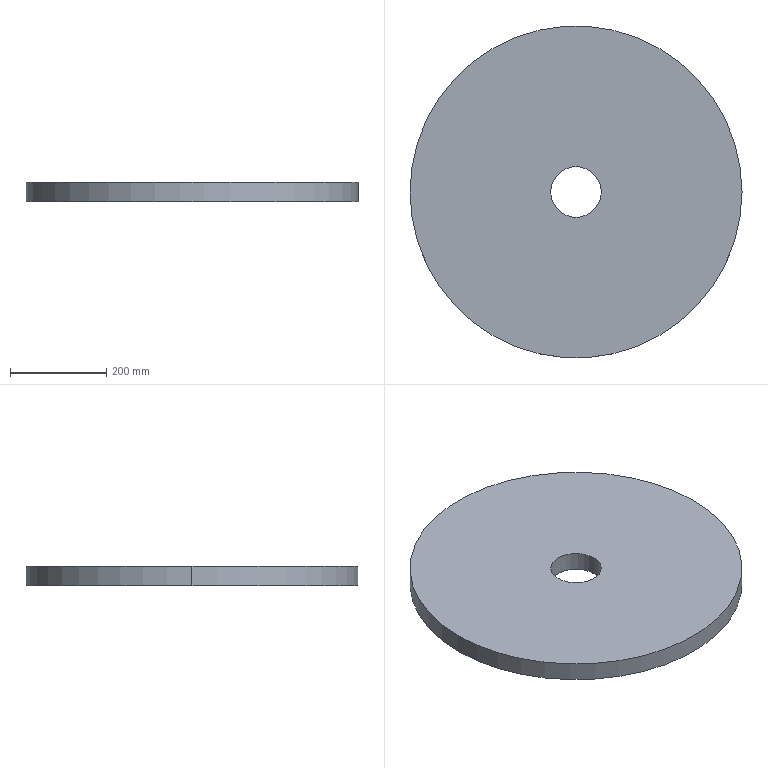Part | SolidWorks | features Extrusion 1, ICE 1 | 1 solid | 6 faces | box 690 x 690 x 40 mm | volume 14610762 mm3 | cylinder 4 | plane 2 | commonest cylinder face diameters 105 x2 690 x2
STEP:
#1=CARTESIAN_POINT('',(-52.5,0.,40.));
#2=VERTEX_POINT('',#1);
#3=CARTESIAN_POINT('',(52.5,0.,40.));
#4=VERTEX_POINT('',#3);
#5=CARTESIAN_POINT('',(0.,0.,40.));
#6=DIRECTION('',(0.,0.,1.));
#7=DIRECTION('',(1.,0.,0.));
#8=AXIS2_PLACEMENT_3D('',#5,#6,#7);
#9=CIRCLE('',#8,52.5);
#10=EDGE_CURVE('',#2,#4,#9,.T.);
#11=ORIENTED_EDGE('',*,*,#10,.T.);
#12=CARTESIAN_POINT('',(52.5,0.,0.));
#13=VERTEX_POINT('',#12);
#14=CARTESIAN_POINT('',(52.5,0.,40.));
#15=DIRECTION('',(0.,0.,-1.));
#16=VECTOR('',#15,1000.);
#17=LINE('',#14,#16);
#18=EDGE_CURVE('',#4,#13,#17,.T.);
#19=ORIENTED_EDGE('',*,*,#18,.T.);
#20=CARTESIAN_POINT('',(-52.5,0.,0.));
#21=VERTEX_POINT('',#20);
#22=CARTESIAN_POINT('',(0.,0.,0.));
#23=DIRECTION('',(0.,0.,-1.));
#24=DIRECTION('',(-1.,0.,0.));
#25=AXIS2_PLACEMENT_3D('',#22,#23,#24);
#26=CIRCLE('',#25,52.5);
#27=EDGE_CURVE('',#13,#21,#26,.T.);
#28=ORIENTED_EDGE('',*,*,#27,.T.);
#29=CARTESIAN_POINT('',(-52.5,0.,40.));
#30=DIRECTION('',(0.,0.,-1.));
#31=VECTOR('',#30,1000.);
#32=LINE('',#29,#31);
#33=EDGE_CURVE('',#2,#21,#32,.T.);
#34=ORIENTED_EDGE('',*,*,#33,.F.);
#35=EDGE_LOOP('',(#11,#19,#28,#34));
#36=FACE_OUTER_BOUND('',#35,.T.);
#37=CARTESIAN_POINT('',(0.,0.,40.));
#38=DIRECTION('',(0.,0.,-1.));
#39=DIRECTION('',(-1.,0.,0.));
#40=AXIS2_PLACEMENT_3D('',#37,#38,#39);
#41=CYLINDRICAL_SURFACE('',#40,52.5);
#42=ADVANCED_FACE('',(#36),#41,.F.);
#43=CARTESIAN_POINT('',(345.,0.,40.));
#44=VERTEX_POINT('',#43);
#45=CARTESIAN_POINT('',(-345.,0.,40.));
#46=VERTEX_POINT('',#45);
#47=CARTESIAN_POINT('',(0.,0.,40.));
#48=DIRECTION('',(0.,0.,1.));
#49=DIRECTION('',(1.,0.,0.));
#50=AXIS2_PLACEMENT_3D('',#47,#48,#49);
#51=CIRCLE('',#50,345.);
#52=EDGE_CURVE('',#44,#46,#51,.T.);
#53=ORIENTED_EDGE('',*,*,#52,.F.);
#54=CARTESIAN_POINT('',(345.,0.,0.));
#55=VERTEX_POINT('',#54);
#56=CARTESIAN_POINT('',(345.,0.,40.));
#57=DIRECTION('',(0.,0.,-1.));
#58=VECTOR('',#57,1000.);
#59=LINE('',#56,#58);
#60=EDGE_CURVE('',#44,#55,#59,.T.);
#61=ORIENTED_EDGE('',*,*,#60,.T.);
#62=CARTESIAN_POINT('',(-345.,0.,0.));
#63=VERTEX_POINT('',#62);
#64=CARTESIAN_POINT('',(0.,0.,0.));
#65=DIRECTION('',(0.,0.,1.));
#66=DIRECTION('',(1.,0.,0.));
#67=AXIS2_PLACEMENT_3D('',#64,#65,#66);
#68=CIRCLE('',#67,345.);
#69=EDGE_CURVE('',#55,#63,#68,.T.);
#70=ORIENTED_EDGE('',*,*,#69,.T.);
#71=CARTESIAN_POINT('',(-345.,0.,40.));
#72=DIRECTION('',(0.,0.,-1.));
#73=VECTOR('',#72,1000.);
#74=LINE('',#71,#73);
#75=EDGE_CURVE('',#46,#63,#74,.T.);
#76=ORIENTED_EDGE('',*,*,#75,.F.);
#77=EDGE_LOOP('',(#53,#61,#70,#76));
#78=FACE_OUTER_BOUND('',#77,.T.);
#79=CARTESIAN_POINT('',(0.,0.,40.));
#80=DIRECTION('',(0.,0.,-1.));
#81=DIRECTION('',(-1.,0.,0.));
#82=AXIS2_PLACEMENT_3D('',#79,#80,#81);
#83=CYLINDRICAL_SURFACE('',#82,345.);
#84=ADVANCED_FACE('',(#78),#83,.T.);
#85=ORIENTED_EDGE('',*,*,#60,.F.);
#86=CARTESIAN_POINT('',(0.,0.,40.));
#87=DIRECTION('',(0.,0.,1.));
#88=DIRECTION('',(1.,0.,0.));
#89=AXIS2_PLACEMENT_3D('',#86,#87,#88);
#90=CIRCLE('',#89,345.);
#91=EDGE_CURVE('',#46,#44,#90,.T.);
#92=ORIENTED_EDGE('',*,*,#91,.F.);
#93=ORIENTED_EDGE('',*,*,#75,.T.);
#94=CARTESIAN_POINT('',(0.,0.,0.));
#95=DIRECTION('',(0.,0.,1.));
#96=DIRECTION('',(1.,0.,0.));
#97=AXIS2_PLACEMENT_3D('',#94,#95,#96);
#98=CIRCLE('',#97,345.);
#99=EDGE_CURVE('',#63,#55,#98,.T.);
#100=ORIENTED_EDGE('',*,*,#99,.T.);
#101=EDGE_LOOP('',(#85,#92,#93,#100));
#102=FACE_OUTER_BOUND('',#101,.T.);
#103=CARTESIAN_POINT('',(0.,0.,40.));
#104=DIRECTION('',(0.,0.,-1.));
#105=DIRECTION('',(-1.,0.,0.));
#106=AXIS2_PLACEMENT_3D('',#103,#104,#105);
#107=CYLINDRICAL_SURFACE('',#106,345.);
#108=ADVANCED_FACE('',(#102),#107,.T.);
#109=ORIENTED_EDGE('',*,*,#10,.F.);
#110=CARTESIAN_POINT('',(0.,0.,40.));
#111=DIRECTION('',(0.,0.,1.));
#112=DIRECTION('',(1.,0.,0.));
#113=AXIS2_PLACEMENT_3D('',#110,#111,#112);
#114=CIRCLE('',#113,52.5);
#115=EDGE_CURVE('',#4,#2,#114,.T.);
#116=ORIENTED_EDGE('',*,*,#115,.F.);
#117=EDGE_LOOP('',(#109,#116));
#118=FACE_BOUND('',#117,.T.);
#119=ORIENTED_EDGE('',*,*,#91,.T.);
#120=ORIENTED_EDGE('',*,*,#52,.T.);
#121=EDGE_LOOP('',(#119,#120));
#122=FACE_OUTER_BOUND('',#121,.T.);
#123=CARTESIAN_POINT('',(0.,0.,40.));
#124=DIRECTION('',(0.,0.,1.));
#125=DIRECTION('',(1.,0.,0.));
#126=AXIS2_PLACEMENT_3D('',#123,#124,#125);
#127=PLANE('',#126);
#128=ADVANCED_FACE('',(#118,#122),#127,.T.);
#129=CARTESIAN_POINT('',(0.,0.,0.));
#130=DIRECTION('',(0.,0.,-1.));
#131=DIRECTION('',(-1.,0.,0.));
#132=AXIS2_PLACEMENT_3D('',#129,#130,#131);
#133=CIRCLE('',#132,52.5);
#134=EDGE_CURVE('',#21,#13,#133,.T.);
#135=ORIENTED_EDGE('',*,*,#134,.F.);
#136=ORIENTED_EDGE('',*,*,#27,.F.);
#137=EDGE_LOOP('',(#135,#136));
#138=FACE_BOUND('',#137,.T.);
#139=ORIENTED_EDGE('',*,*,#99,.F.);
#140=ORIENTED_EDGE('',*,*,#69,.F.);
#141=EDGE_LOOP('',(#139,#140));
#142=FACE_OUTER_BOUND('',#141,.T.);
#143=CARTESIAN_POINT('',(0.,0.,0.));
#144=DIRECTION('',(0.,0.,1.));
#145=DIRECTION('',(1.,0.,0.));
#146=AXIS2_PLACEMENT_3D('',#143,#144,#145);
#147=PLANE('',#146);
#148=ADVANCED_FACE('',(#138,#142),#147,.F.);
#149=ORIENTED_EDGE('',*,*,#18,.F.);
#150=ORIENTED_EDGE('',*,*,#115,.T.);
#151=ORIENTED_EDGE('',*,*,#33,.T.);
#152=ORIENTED_EDGE('',*,*,#134,.T.);
#153=EDGE_LOOP('',(#149,#150,#151,#152));
#154=FACE_OUTER_BOUND('',#153,.T.);
#155=CARTESIAN_POINT('',(0.,0.,40.));
#156=DIRECTION('',(0.,0.,-1.));
#157=DIRECTION('',(-1.,0.,0.));
#158=AXIS2_PLACEMENT_3D('',#155,#156,#157);
#159=CYLINDRICAL_SURFACE('',#158,52.5);
#160=ADVANCED_FACE('',(#154),#159,.F.);
#161=CLOSED_SHELL('',(#42,#84,#108,#128,#148,#160));
#162=MANIFOLD_SOLID_BREP('',#161);
#163=CARTESIAN_POINT('',(0.,0.,0.));
#164=DIRECTION('',(0.,0.,1.));
#165=DIRECTION('',(1.,0.,0.));
#166=AXIS2_PLACEMENT_3D('',#163,#164,#165);
#167=(LENGTH_UNIT()NAMED_UNIT(*)SI_UNIT(.MILLI.,.METRE.));
#168=UNCERTAINTY_MEASURE_WITH_UNIT(LENGTH_MEASURE(0.00001),#167,'','');
#169=(NAMED_UNIT(*)PLANE_ANGLE_UNIT()SI_UNIT($,.RADIAN.));
#170=(NAMED_UNIT(*)SI_UNIT($,.STERADIAN.)SOLID_ANGLE_UNIT());
#171=(GEOMETRIC_REPRESENTATION_CONTEXT(3)GLOBAL_UNCERTAINTY_ASSIGNED_CONTEXT((#168))GLOBAL_UNIT_ASSIGNED_CONTEXT((#167,#169,#170))REPRESENTATION_CONTEXT('',''));
#172=ADVANCED_BREP_SHAPE_REPRESENTATION('',(#162,#166),#171);